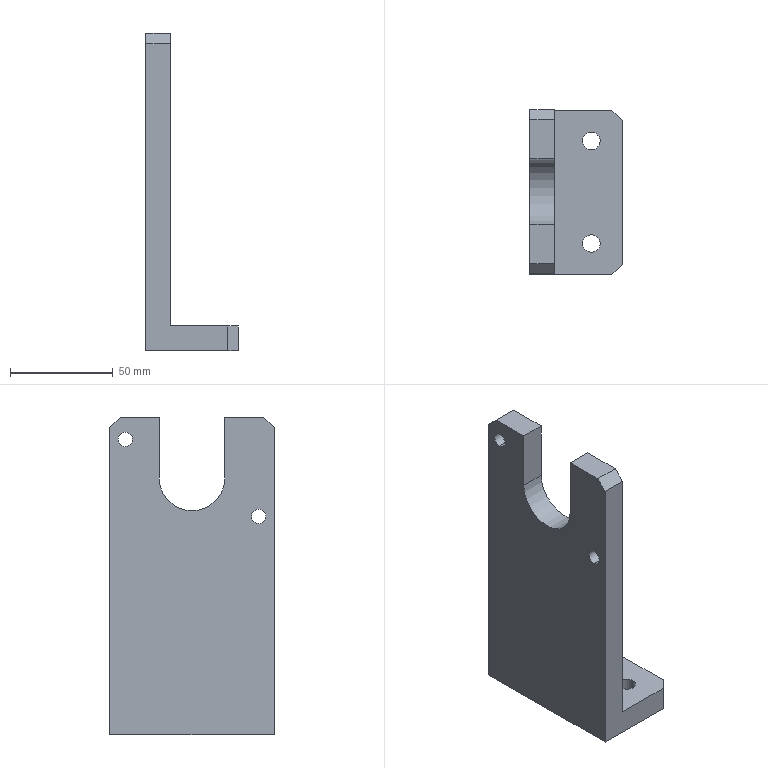Part | SolidWorks | features BaseBody 1 | 1 solid | 24 faces | box 45 x 80 x 154.5 mm | volume 160965 mm3 | plane 15 | cylinder 9 | commonest cylinder face diameters 6.985 x4 8.5 x4 32 x1
STEP:
#1=CARTESIAN_POINT('',(0.,32.476,220.743));
#2=VERTEX_POINT('',#1);
#3=CARTESIAN_POINT('',(0.,32.476,213.757));
#4=VERTEX_POINT('',#3);
#5=CARTESIAN_POINT('',(0.,32.476,217.25));
#6=DIRECTION('',(1.,0.,0.));
#7=DIRECTION('',(0.,0.,1.));
#8=AXIS2_PLACEMENT_3D('',#5,#6,#7);
#9=CIRCLE('',#8,3.493);
#10=EDGE_CURVE('',#2,#4,#9,.T.);
#11=ORIENTED_EDGE('',*,*,#10,.F.);
#12=CARTESIAN_POINT('',(12.,32.476,220.743));
#13=VERTEX_POINT('',#12);
#14=CARTESIAN_POINT('',(0.,32.476,220.743));
#15=DIRECTION('',(1.,0.,0.));
#16=VECTOR('',#15,1000.);
#17=LINE('',#14,#16);
#18=EDGE_CURVE('',#2,#13,#17,.T.);
#19=ORIENTED_EDGE('',*,*,#18,.T.);
#20=CARTESIAN_POINT('',(12.,32.476,213.757));
#21=VERTEX_POINT('',#20);
#22=CARTESIAN_POINT('',(12.,32.476,217.25));
#23=DIRECTION('',(-1.,0.,0.));
#24=DIRECTION('',(0.,0.,-1.));
#25=AXIS2_PLACEMENT_3D('',#22,#23,#24);
#26=CIRCLE('',#25,3.493);
#27=EDGE_CURVE('',#21,#13,#26,.T.);
#28=ORIENTED_EDGE('',*,*,#27,.F.);
#29=CARTESIAN_POINT('',(0.,32.476,213.757));
#30=DIRECTION('',(1.,0.,0.));
#31=VECTOR('',#30,1000.);
#32=LINE('',#29,#31);
#33=EDGE_CURVE('',#4,#21,#32,.T.);
#34=ORIENTED_EDGE('',*,*,#33,.F.);
#35=EDGE_LOOP('',(#11,#19,#28,#34));
#36=FACE_OUTER_BOUND('',#35,.T.);
#37=CARTESIAN_POINT('',(0.,32.476,217.25));
#38=DIRECTION('',(1.,0.,0.));
#39=DIRECTION('',(0.,0.,-1.));
#40=AXIS2_PLACEMENT_3D('',#37,#38,#39);
#41=CYLINDRICAL_SURFACE('',#40,3.493);
#42=ADVANCED_FACE('',(#36),#41,.F.);
#43=CARTESIAN_POINT('',(0.,-32.476,183.243));
#44=VERTEX_POINT('',#43);
#45=CARTESIAN_POINT('',(0.,-32.476,176.257));
#46=VERTEX_POINT('',#45);
#47=CARTESIAN_POINT('',(0.,-32.476,179.75));
#48=DIRECTION('',(1.,0.,0.));
#49=DIRECTION('',(0.,0.,1.));
#50=AXIS2_PLACEMENT_3D('',#47,#48,#49);
#51=CIRCLE('',#50,3.493);
#52=EDGE_CURVE('',#44,#46,#51,.T.);
#53=ORIENTED_EDGE('',*,*,#52,.F.);
#54=CARTESIAN_POINT('',(12.,-32.476,183.243));
#55=VERTEX_POINT('',#54);
#56=CARTESIAN_POINT('',(0.,-32.476,183.243));
#57=DIRECTION('',(1.,0.,0.));
#58=VECTOR('',#57,1000.);
#59=LINE('',#56,#58);
#60=EDGE_CURVE('',#44,#55,#59,.T.);
#61=ORIENTED_EDGE('',*,*,#60,.T.);
#62=CARTESIAN_POINT('',(12.,-32.476,176.257));
#63=VERTEX_POINT('',#62);
#64=CARTESIAN_POINT('',(12.,-32.476,179.75));
#65=DIRECTION('',(-1.,0.,0.));
#66=DIRECTION('',(0.,0.,-1.));
#67=AXIS2_PLACEMENT_3D('',#64,#65,#66);
#68=CIRCLE('',#67,3.493);
#69=EDGE_CURVE('',#63,#55,#68,.T.);
#70=ORIENTED_EDGE('',*,*,#69,.F.);
#71=CARTESIAN_POINT('',(0.,-32.476,176.257));
#72=DIRECTION('',(1.,0.,0.));
#73=VECTOR('',#72,1000.);
#74=LINE('',#71,#73);
#75=EDGE_CURVE('',#46,#63,#74,.T.);
#76=ORIENTED_EDGE('',*,*,#75,.F.);
#77=EDGE_LOOP('',(#53,#61,#70,#76));
#78=FACE_OUTER_BOUND('',#77,.T.);
#79=CARTESIAN_POINT('',(0.,-32.476,179.75));
#80=DIRECTION('',(1.,0.,0.));
#81=DIRECTION('',(0.,0.,-1.));
#82=AXIS2_PLACEMENT_3D('',#79,#80,#81);
#83=CYLINDRICAL_SURFACE('',#82,3.493);
#84=ADVANCED_FACE('',(#78),#83,.F.);
#85=CARTESIAN_POINT('',(34.25,25.,85.5));
#86=VERTEX_POINT('',#85);
#87=CARTESIAN_POINT('',(25.75,25.,85.5));
#88=VERTEX_POINT('',#87);
#89=CARTESIAN_POINT('',(30.,25.,85.5));
#90=DIRECTION('',(0.,0.,-1.));
#91=DIRECTION('',(-1.,0.,0.));
#92=AXIS2_PLACEMENT_3D('',#89,#90,#91);
#93=CIRCLE('',#92,4.25);
#94=EDGE_CURVE('',#86,#88,#93,.T.);
#95=ORIENTED_EDGE('',*,*,#94,.F.);
#96=CARTESIAN_POINT('',(34.25,25.,73.5));
#97=VERTEX_POINT('',#96);
#98=CARTESIAN_POINT('',(34.25,25.,85.5));
#99=DIRECTION('',(0.,0.,-1.));
#100=VECTOR('',#99,1000.);
#101=LINE('',#98,#100);
#102=EDGE_CURVE('',#86,#97,#101,.T.);
#103=ORIENTED_EDGE('',*,*,#102,.T.);
#104=CARTESIAN_POINT('',(25.75,25.,73.5));
#105=VERTEX_POINT('',#104);
#106=CARTESIAN_POINT('',(30.,25.,73.5));
#107=DIRECTION('',(0.,0.,1.));
#108=DIRECTION('',(-1.,0.,0.));
#109=AXIS2_PLACEMENT_3D('',#106,#107,#108);
#110=CIRCLE('',#109,4.25);
#111=EDGE_CURVE('',#105,#97,#110,.T.);
#112=ORIENTED_EDGE('',*,*,#111,.F.);
#113=CARTESIAN_POINT('',(25.75,25.,85.5));
#114=DIRECTION('',(0.,0.,-1.));
#115=VECTOR('',#114,1000.);
#116=LINE('',#113,#115);
#117=EDGE_CURVE('',#88,#105,#116,.T.);
#118=ORIENTED_EDGE('',*,*,#117,.F.);
#119=EDGE_LOOP('',(#95,#103,#112,#118));
#120=FACE_OUTER_BOUND('',#119,.T.);
#121=CARTESIAN_POINT('',(30.,25.,85.5));
#122=DIRECTION('',(0.,0.,-1.));
#123=DIRECTION('',(-1.,0.,0.));
#124=AXIS2_PLACEMENT_3D('',#121,#122,#123);
#125=CYLINDRICAL_SURFACE('',#124,4.25);
#126=ADVANCED_FACE('',(#120),#125,.F.);
#127=CARTESIAN_POINT('',(34.25,-25.,85.5));
#128=VERTEX_POINT('',#127);
#129=CARTESIAN_POINT('',(25.75,-25.,85.5));
#130=VERTEX_POINT('',#129);
#131=CARTESIAN_POINT('',(30.,-25.,85.5));
#132=DIRECTION('',(0.,0.,-1.));
#133=DIRECTION('',(-1.,0.,0.));
#134=AXIS2_PLACEMENT_3D('',#131,#132,#133);
#135=CIRCLE('',#134,4.25);
#136=EDGE_CURVE('',#128,#130,#135,.T.);
#137=ORIENTED_EDGE('',*,*,#136,.F.);
#138=CARTESIAN_POINT('',(34.25,-25.,73.5));
#139=VERTEX_POINT('',#138);
#140=CARTESIAN_POINT('',(34.25,-25.,85.5));
#141=DIRECTION('',(0.,0.,-1.));
#142=VECTOR('',#141,1000.);
#143=LINE('',#140,#142);
#144=EDGE_CURVE('',#128,#139,#143,.T.);
#145=ORIENTED_EDGE('',*,*,#144,.T.);
#146=CARTESIAN_POINT('',(25.75,-25.,73.5));
#147=VERTEX_POINT('',#146);
#148=CARTESIAN_POINT('',(30.,-25.,73.5));
#149=DIRECTION('',(0.,0.,1.));
#150=DIRECTION('',(-1.,0.,0.));
#151=AXIS2_PLACEMENT_3D('',#148,#149,#150);
#152=CIRCLE('',#151,4.25);
#153=EDGE_CURVE('',#147,#139,#152,.T.);
#154=ORIENTED_EDGE('',*,*,#153,.F.);
#155=CARTESIAN_POINT('',(25.75,-25.,85.5));
#156=DIRECTION('',(0.,0.,-1.));
#157=VECTOR('',#156,1000.);
#158=LINE('',#155,#157);
#159=EDGE_CURVE('',#130,#147,#158,.T.);
#160=ORIENTED_EDGE('',*,*,#159,.F.);
#161=EDGE_LOOP('',(#137,#145,#154,#160));
#162=FACE_OUTER_BOUND('',#161,.T.);
#163=CARTESIAN_POINT('',(30.,-25.,85.5));
#164=DIRECTION('',(0.,0.,-1.));
#165=DIRECTION('',(-1.,0.,0.));
#166=AXIS2_PLACEMENT_3D('',#163,#164,#165);
#167=CYLINDRICAL_SURFACE('',#166,4.25);
#168=ADVANCED_FACE('',(#162),#167,.F.);
#169=CARTESIAN_POINT('',(0.,40.,223.));
#170=VERTEX_POINT('',#169);
#171=CARTESIAN_POINT('',(0.,40.,73.5));
#172=VERTEX_POINT('',#171);
#173=CARTESIAN_POINT('',(0.,40.,133.5));
#174=DIRECTION('',(0.,0.,-1.));
#175=VECTOR('',#174,1000.);
#176=LINE('',#173,#175);
#177=EDGE_CURVE('',#170,#172,#176,.T.);
#178=ORIENTED_EDGE('',*,*,#177,.T.);
#179=CARTESIAN_POINT('',(0.,-40.,73.5));
#180=VERTEX_POINT('',#179);
#181=CARTESIAN_POINT('',(0.,-42.5,73.5));
#182=DIRECTION('',(0.,-1.,0.));
#183=VECTOR('',#182,1000.);
#184=LINE('',#181,#183);
#185=EDGE_CURVE('',#172,#180,#184,.T.);
#186=ORIENTED_EDGE('',*,*,#185,.T.);
#187=CARTESIAN_POINT('',(0.,-40.,223.));
#188=VERTEX_POINT('',#187);
#189=CARTESIAN_POINT('',(0.,-40.,133.5));
#190=DIRECTION('',(0.,0.,1.));
#191=VECTOR('',#190,1000.);
#192=LINE('',#189,#191);
#193=EDGE_CURVE('',#180,#188,#192,.T.);
#194=ORIENTED_EDGE('',*,*,#193,.T.);
#195=CARTESIAN_POINT('',(0.,-35.,228.));
#196=VERTEX_POINT('',#195);
#197=CARTESIAN_POINT('',(0.,-84.75,178.25));
#198=DIRECTION('',(0.,0.7071,0.7071));
#199=VECTOR('',#198,1000.);
#200=LINE('',#197,#199);
#201=EDGE_CURVE('',#188,#196,#200,.T.);
#202=ORIENTED_EDGE('',*,*,#201,.T.);
#203=CARTESIAN_POINT('',(0.,-16.,228.));
#204=VERTEX_POINT('',#203);
#205=CARTESIAN_POINT('',(0.,-42.5,228.));
#206=DIRECTION('',(0.,1.,0.));
#207=VECTOR('',#206,1000.);
#208=LINE('',#205,#207);
#209=EDGE_CURVE('',#196,#204,#208,.T.);
#210=ORIENTED_EDGE('',*,*,#209,.T.);
#211=CARTESIAN_POINT('',(0.,-16.,198.5));
#212=VERTEX_POINT('',#211);
#213=CARTESIAN_POINT('',(0.,-16.,133.5));
#214=DIRECTION('',(0.,0.,-1.));
#215=VECTOR('',#214,1000.);
#216=LINE('',#213,#215);
#217=EDGE_CURVE('',#204,#212,#216,.T.);
#218=ORIENTED_EDGE('',*,*,#217,.T.);
#219=CARTESIAN_POINT('',(0.,16.,198.5));
#220=VERTEX_POINT('',#219);
#221=CARTESIAN_POINT('',(0.,0.,198.5));
#222=DIRECTION('',(1.,0.,0.));
#223=DIRECTION('',(0.,0.,1.));
#224=AXIS2_PLACEMENT_3D('',#221,#222,#223);
#225=CIRCLE('',#224,16.);
#226=EDGE_CURVE('',#212,#220,#225,.T.);
#227=ORIENTED_EDGE('',*,*,#226,.T.);
#228=CARTESIAN_POINT('',(0.,16.,228.));
#229=VERTEX_POINT('',#228);
#230=CARTESIAN_POINT('',(0.,16.,133.5));
#231=DIRECTION('',(0.,0.,1.));
#232=VECTOR('',#231,1000.);
#233=LINE('',#230,#232);
#234=EDGE_CURVE('',#220,#229,#233,.T.);
#235=ORIENTED_EDGE('',*,*,#234,.T.);
#236=CARTESIAN_POINT('',(0.,35.,228.));
#237=VERTEX_POINT('',#236);
#238=CARTESIAN_POINT('',(0.,-42.5,228.));
#239=DIRECTION('',(0.,1.,0.));
#240=VECTOR('',#239,1000.);
#241=LINE('',#238,#240);
#242=EDGE_CURVE('',#229,#237,#241,.T.);
#243=ORIENTED_EDGE('',*,*,#242,.T.);
#244=CARTESIAN_POINT('',(0.,40.,223.));
#245=DIRECTION('',(0.,0.7071,-0.7071));
#246=VECTOR('',#245,1000.);
#247=LINE('',#244,#246);
#248=EDGE_CURVE('',#237,#170,#247,.T.);
#249=ORIENTED_EDGE('',*,*,#248,.T.);
#250=EDGE_LOOP('',(#178,#186,#194,#202,#210,#218,#227,#235,#243,#249));
#251=FACE_OUTER_BOUND('',#250,.T.);
#252=CARTESIAN_POINT('',(0.,32.476,217.25));
#253=DIRECTION('',(1.,0.,0.));
#254=DIRECTION('',(0.,0.,1.));
#255=AXIS2_PLACEMENT_3D('',#252,#253,#254);
#256=CIRCLE('',#255,3.493);
#257=EDGE_CURVE('',#4,#2,#256,.T.);
#258=ORIENTED_EDGE('',*,*,#257,.T.);
#259=ORIENTED_EDGE('',*,*,#10,.T.);
#260=EDGE_LOOP('',(#258,#259));
#261=FACE_BOUND('',#260,.T.);
#262=CARTESIAN_POINT('',(0.,-32.476,179.75));
#263=DIRECTION('',(1.,0.,0.));
#264=DIRECTION('',(0.,0.,1.));
#265=AXIS2_PLACEMENT_3D('',#262,#263,#264);
#266=CIRCLE('',#265,3.493);
#267=EDGE_CURVE('',#46,#44,#266,.T.);
#268=ORIENTED_EDGE('',*,*,#267,.T.);
#269=ORIENTED_EDGE('',*,*,#52,.T.);
#270=EDGE_LOOP('',(#268,#269));
#271=FACE_BOUND('',#270,.T.);
#272=CARTESIAN_POINT('',(0.,-42.5,133.5));
#273=DIRECTION('',(-1.,0.,0.));
#274=DIRECTION('',(0.,0.,1.));
#275=AXIS2_PLACEMENT_3D('',#272,#273,#274);
#276=PLANE('',#275);
#277=ADVANCED_FACE('',(#251,#261,#271),#276,.T.);
#278=CARTESIAN_POINT('',(40.,-40.,73.5));
#279=VERTEX_POINT('',#278);
#280=CARTESIAN_POINT('',(0.,-40.,73.5));
#281=DIRECTION('',(-1.,0.,0.));
#282=VECTOR('',#281,1000.);
#283=LINE('',#280,#282);
#284=EDGE_CURVE('',#279,#180,#283,.T.);
#285=ORIENTED_EDGE('',*,*,#284,.T.);
#286=ORIENTED_EDGE('',*,*,#185,.F.);
#287=CARTESIAN_POINT('',(40.,40.,73.5));
#288=VERTEX_POINT('',#287);
#289=CARTESIAN_POINT('',(45.,40.,73.5));
#290=DIRECTION('',(1.,0.,0.));
#291=VECTOR('',#290,1000.);
#292=LINE('',#289,#291);
#293=EDGE_CURVE('',#172,#288,#292,.T.);
#294=ORIENTED_EDGE('',*,*,#293,.T.);
#295=CARTESIAN_POINT('',(45.,35.,73.5));
#296=VERTEX_POINT('',#295);
#297=CARTESIAN_POINT('',(40.,40.,73.5));
#298=DIRECTION('',(0.7071,-0.7071,0.));
#299=VECTOR('',#298,1000.);
#300=LINE('',#297,#299);
#301=EDGE_CURVE('',#288,#296,#300,.T.);
#302=ORIENTED_EDGE('',*,*,#301,.T.);
#303=CARTESIAN_POINT('',(45.,-35.,73.5));
#304=VERTEX_POINT('',#303);
#305=CARTESIAN_POINT('',(45.,-42.5,73.5));
#306=DIRECTION('',(0.,-1.,0.));
#307=VECTOR('',#306,1000.);
#308=LINE('',#305,#307);
#309=EDGE_CURVE('',#296,#304,#308,.T.);
#310=ORIENTED_EDGE('',*,*,#309,.T.);
#311=CARTESIAN_POINT('',(45.,-35.,73.5));
#312=DIRECTION('',(-0.7071,-0.7071,0.));
#313=VECTOR('',#312,1000.);
#314=LINE('',#311,#313);
#315=EDGE_CURVE('',#304,#279,#314,.T.);
#316=ORIENTED_EDGE('',*,*,#315,.T.);
#317=EDGE_LOOP('',(#285,#286,#294,#302,#310,#316));
#318=FACE_OUTER_BOUND('',#317,.T.);
#319=ORIENTED_EDGE('',*,*,#111,.T.);
#320=CARTESIAN_POINT('',(30.,25.,73.5));
#321=DIRECTION('',(0.,0.,1.));
#322=DIRECTION('',(-1.,0.,0.));
#323=AXIS2_PLACEMENT_3D('',#320,#321,#322);
#324=CIRCLE('',#323,4.25);
#325=EDGE_CURVE('',#97,#105,#324,.T.);
#326=ORIENTED_EDGE('',*,*,#325,.T.);
#327=EDGE_LOOP('',(#319,#326));
#328=FACE_BOUND('',#327,.T.);
#329=ORIENTED_EDGE('',*,*,#153,.T.);
#330=CARTESIAN_POINT('',(30.,-25.,73.5));
#331=DIRECTION('',(0.,0.,1.));
#332=DIRECTION('',(-1.,0.,0.));
#333=AXIS2_PLACEMENT_3D('',#330,#331,#332);
#334=CIRCLE('',#333,4.25);
#335=EDGE_CURVE('',#139,#147,#334,.T.);
#336=ORIENTED_EDGE('',*,*,#335,.T.);
#337=EDGE_LOOP('',(#329,#336));
#338=FACE_BOUND('',#337,.T.);
#339=CARTESIAN_POINT('',(45.,-42.5,73.5));
#340=DIRECTION('',(0.,0.,-1.));
#341=DIRECTION('',(-1.,0.,0.));
#342=AXIS2_PLACEMENT_3D('',#339,#340,#341);
#343=PLANE('',#342);
#344=ADVANCED_FACE('',(#318,#328,#338),#343,.T.);
#345=CARTESIAN_POINT('',(12.,40.,223.));
#346=VERTEX_POINT('',#345);
#347=CARTESIAN_POINT('',(0.,40.,223.));
#348=DIRECTION('',(1.,0.,0.));
#349=VECTOR('',#348,1000.);
#350=LINE('',#347,#349);
#351=EDGE_CURVE('',#170,#346,#350,.T.);
#352=ORIENTED_EDGE('',*,*,#351,.T.);
#353=CARTESIAN_POINT('',(12.,40.,85.5));
#354=VERTEX_POINT('',#353);
#355=CARTESIAN_POINT('',(12.,40.,72.));
#356=DIRECTION('',(0.,0.,-1.));
#357=VECTOR('',#356,1000.);
#358=LINE('',#355,#357);
#359=EDGE_CURVE('',#346,#354,#358,.T.);
#360=ORIENTED_EDGE('',*,*,#359,.T.);
#361=CARTESIAN_POINT('',(40.,40.,85.5));
#362=VERTEX_POINT('',#361);
#363=CARTESIAN_POINT('',(0.,40.,85.5));
#364=DIRECTION('',(1.,0.,0.));
#365=VECTOR('',#364,1000.);
#366=LINE('',#363,#365);
#367=EDGE_CURVE('',#354,#362,#366,.T.);
#368=ORIENTED_EDGE('',*,*,#367,.T.);
#369=CARTESIAN_POINT('',(40.,40.,145.5));
#370=DIRECTION('',(0.,0.,-1.));
#371=VECTOR('',#370,1000.);
#372=LINE('',#369,#371);
#373=EDGE_CURVE('',#362,#288,#372,.T.);
#374=ORIENTED_EDGE('',*,*,#373,.T.);
#375=ORIENTED_EDGE('',*,*,#293,.F.);
#376=ORIENTED_EDGE('',*,*,#177,.F.);
#377=EDGE_LOOP('',(#352,#360,#368,#374,#375,#376));
#378=FACE_OUTER_BOUND('',#377,.T.);
#379=CARTESIAN_POINT('',(0.,40.,72.));
#380=DIRECTION('',(0.,1.,0.));
#381=DIRECTION('',(0.,0.,1.));
#382=AXIS2_PLACEMENT_3D('',#379,#380,#381);
#383=PLANE('',#382);
#384=ADVANCED_FACE('',(#378),#383,.T.);
#385=CARTESIAN_POINT('',(12.,35.,228.));
#386=VERTEX_POINT('',#385);
#387=CARTESIAN_POINT('',(0.,35.,228.));
#388=DIRECTION('',(-1.,0.,0.));
#389=VECTOR('',#388,1000.);
#390=LINE('',#387,#389);
#391=EDGE_CURVE('',#386,#237,#390,.T.);
#392=ORIENTED_EDGE('',*,*,#391,.F.);
#393=CARTESIAN_POINT('',(12.,40.,223.));
#394=DIRECTION('',(0.,-0.7071,0.7071));
#395=VECTOR('',#394,1000.);
#396=LINE('',#393,#395);
#397=EDGE_CURVE('',#346,#386,#396,.T.);
#398=ORIENTED_EDGE('',*,*,#397,.F.);
#399=ORIENTED_EDGE('',*,*,#351,.F.);
#400=ORIENTED_EDGE('',*,*,#248,.F.);
#401=EDGE_LOOP('',(#392,#398,#399,#400));
#402=FACE_OUTER_BOUND('',#401,.T.);
#403=CARTESIAN_POINT('',(0.,40.,223.));
#404=DIRECTION('',(0.,-0.7071,-0.7071));
#405=DIRECTION('',(0.,0.7071,-0.7071));
#406=AXIS2_PLACEMENT_3D('',#403,#404,#405);
#407=PLANE('',#406);
#408=ADVANCED_FACE('',(#402),#407,.F.);
#409=ORIENTED_EDGE('',*,*,#242,.F.);
#410=CARTESIAN_POINT('',(12.,16.,228.));
#411=VERTEX_POINT('',#410);
#412=CARTESIAN_POINT('',(0.,16.,228.));
#413=DIRECTION('',(1.,0.,0.));
#414=VECTOR('',#413,1000.);
#415=LINE('',#412,#414);
#416=EDGE_CURVE('',#229,#411,#415,.T.);
#417=ORIENTED_EDGE('',*,*,#416,.T.);
#418=CARTESIAN_POINT('',(12.,-42.5,228.));
#419=DIRECTION('',(0.,1.,0.));
#420=VECTOR('',#419,1000.);
#421=LINE('',#418,#420);
#422=EDGE_CURVE('',#411,#386,#421,.T.);
#423=ORIENTED_EDGE('',*,*,#422,.T.);
#424=ORIENTED_EDGE('',*,*,#391,.T.);
#425=EDGE_LOOP('',(#409,#417,#423,#424));
#426=FACE_OUTER_BOUND('',#425,.T.);
#427=CARTESIAN_POINT('',(0.,-42.5,228.));
#428=DIRECTION('',(0.,0.,1.));
#429=DIRECTION('',(1.,0.,0.));
#430=AXIS2_PLACEMENT_3D('',#427,#428,#429);
#431=PLANE('',#430);
#432=ADVANCED_FACE('',(#426),#431,.T.);
#433=CARTESIAN_POINT('',(12.,16.,198.5));
#434=VERTEX_POINT('',#433);
#435=CARTESIAN_POINT('',(30.,16.,198.5));
#436=DIRECTION('',(1.,0.,0.));
#437=VECTOR('',#436,1000.);
#438=LINE('',#435,#437);
#439=EDGE_CURVE('',#220,#434,#438,.T.);
#440=ORIENTED_EDGE('',*,*,#439,.T.);
#441=CARTESIAN_POINT('',(12.,16.,198.5));
#442=DIRECTION('',(0.,0.,1.));
#443=VECTOR('',#442,1000.);
#444=LINE('',#441,#443);
#445=EDGE_CURVE('',#434,#411,#444,.T.);
#446=ORIENTED_EDGE('',*,*,#445,.T.);
#447=ORIENTED_EDGE('',*,*,#416,.F.);
#448=ORIENTED_EDGE('',*,*,#234,.F.);
#449=EDGE_LOOP('',(#440,#446,#447,#448));
#450=FACE_OUTER_BOUND('',#449,.T.);
#451=CARTESIAN_POINT('',(30.,16.,198.5));
#452=DIRECTION('',(0.,-1.,0.));
#453=DIRECTION('',(0.,0.,-1.));
#454=AXIS2_PLACEMENT_3D('',#451,#452,#453);
#455=PLANE('',#454);
#456=ADVANCED_FACE('',(#450),#455,.T.);
#457=ORIENTED_EDGE('',*,*,#226,.F.);
#458=CARTESIAN_POINT('',(12.,-16.,198.5));
#459=VERTEX_POINT('',#458);
#460=CARTESIAN_POINT('',(30.,-16.,198.5));
#461=DIRECTION('',(-1.,0.,0.));
#462=VECTOR('',#461,1000.);
#463=LINE('',#460,#462);
#464=EDGE_CURVE('',#459,#212,#463,.T.);
#465=ORIENTED_EDGE('',*,*,#464,.F.);
#466=CARTESIAN_POINT('',(12.,0.,198.5));
#467=DIRECTION('',(-1.,0.,0.));
#468=DIRECTION('',(0.,0.,1.));
#469=AXIS2_PLACEMENT_3D('',#466,#467,#468);
#470=CIRCLE('',#469,16.);
#471=EDGE_CURVE('',#434,#459,#470,.T.);
#472=ORIENTED_EDGE('',*,*,#471,.F.);
#473=ORIENTED_EDGE('',*,*,#439,.F.);
#474=EDGE_LOOP('',(#457,#465,#472,#473));
#475=FACE_OUTER_BOUND('',#474,.T.);
#476=CARTESIAN_POINT('',(30.,0.,198.5));
#477=DIRECTION('',(-1.,0.,0.));
#478=DIRECTION('',(0.,0.,1.));
#479=AXIS2_PLACEMENT_3D('',#476,#477,#478);
#480=CYLINDRICAL_SURFACE('',#479,16.);
#481=ADVANCED_FACE('',(#475),#480,.F.);
#482=CARTESIAN_POINT('',(12.,-16.,228.));
#483=VERTEX_POINT('',#482);
#484=CARTESIAN_POINT('',(30.,-16.,228.));
#485=DIRECTION('',(1.,0.,0.));
#486=VECTOR('',#485,1000.);
#487=LINE('',#484,#486);
#488=EDGE_CURVE('',#204,#483,#487,.T.);
#489=ORIENTED_EDGE('',*,*,#488,.T.);
#490=CARTESIAN_POINT('',(12.,-16.,228.));
#491=DIRECTION('',(0.,0.,-1.));
#492=VECTOR('',#491,1000.);
#493=LINE('',#490,#492);
#494=EDGE_CURVE('',#483,#459,#493,.T.);
#495=ORIENTED_EDGE('',*,*,#494,.T.);
#496=ORIENTED_EDGE('',*,*,#464,.T.);
#497=ORIENTED_EDGE('',*,*,#217,.F.);
#498=EDGE_LOOP('',(#489,#495,#496,#497));
#499=FACE_OUTER_BOUND('',#498,.T.);
#500=CARTESIAN_POINT('',(30.,-16.,228.));
#501=DIRECTION('',(0.,1.,0.));
#502=DIRECTION('',(0.,0.,1.));
#503=AXIS2_PLACEMENT_3D('',#500,#501,#502);
#504=PLANE('',#503);
#505=ADVANCED_FACE('',(#499),#504,.T.);
#506=CARTESIAN_POINT('',(12.,-35.,228.));
#507=VERTEX_POINT('',#506);
#508=CARTESIAN_POINT('',(12.,-42.5,228.));
#509=DIRECTION('',(0.,1.,0.));
#510=VECTOR('',#509,1000.);
#511=LINE('',#508,#510);
#512=EDGE_CURVE('',#507,#483,#511,.T.);
#513=ORIENTED_EDGE('',*,*,#512,.T.);
#514=ORIENTED_EDGE('',*,*,#488,.F.);
#515=ORIENTED_EDGE('',*,*,#209,.F.);
#516=CARTESIAN_POINT('',(0.,-35.,228.));
#517=DIRECTION('',(1.,0.,0.));
#518=VECTOR('',#517,1000.);
#519=LINE('',#516,#518);
#520=EDGE_CURVE('',#196,#507,#519,.T.);
#521=ORIENTED_EDGE('',*,*,#520,.T.);
#522=EDGE_LOOP('',(#513,#514,#515,#521));
#523=FACE_OUTER_BOUND('',#522,.T.);
#524=CARTESIAN_POINT('',(0.,-42.5,228.));
#525=DIRECTION('',(0.,0.,1.));
#526=DIRECTION('',(1.,0.,0.));
#527=AXIS2_PLACEMENT_3D('',#524,#525,#526);
#528=PLANE('',#527);
#529=ADVANCED_FACE('',(#523),#528,.T.);
#530=CARTESIAN_POINT('',(12.,-40.,223.));
#531=VERTEX_POINT('',#530);
#532=CARTESIAN_POINT('',(12.,-35.,228.));
#533=DIRECTION('',(0.,0.7071,0.7071));
#534=VECTOR('',#533,1000.);
#535=LINE('',#532,#534);
#536=EDGE_CURVE('',#531,#507,#535,.T.);
#537=ORIENTED_EDGE('',*,*,#536,.T.);
#538=ORIENTED_EDGE('',*,*,#520,.F.);
#539=ORIENTED_EDGE('',*,*,#201,.F.);
#540=CARTESIAN_POINT('',(0.,-40.,223.));
#541=DIRECTION('',(1.,0.,0.));
#542=VECTOR('',#541,1000.);
#543=LINE('',#540,#542);
#544=EDGE_CURVE('',#188,#531,#543,.T.);
#545=ORIENTED_EDGE('',*,*,#544,.T.);
#546=EDGE_LOOP('',(#537,#538,#539,#545));
#547=FACE_OUTER_BOUND('',#546,.T.);
#548=CARTESIAN_POINT('',(0.,-35.,228.));
#549=DIRECTION('',(0.,-0.7071,0.7071));
#550=DIRECTION('',(0.,-0.7071,-0.7071));
#551=AXIS2_PLACEMENT_3D('',#548,#549,#550);
#552=PLANE('',#551);
#553=ADVANCED_FACE('',(#547),#552,.T.);
#554=CARTESIAN_POINT('',(40.,-40.,85.5));
#555=VERTEX_POINT('',#554);
#556=CARTESIAN_POINT('',(40.,-40.,135.5));
#557=DIRECTION('',(0.,0.,-1.));
#558=VECTOR('',#557,1000.);
#559=LINE('',#556,#558);
#560=EDGE_CURVE('',#555,#279,#559,.T.);
#561=ORIENTED_EDGE('',*,*,#560,.F.);
#562=CARTESIAN_POINT('',(12.,-40.,85.5));
#563=VERTEX_POINT('',#562);
#564=CARTESIAN_POINT('',(0.,-40.,85.5));
#565=DIRECTION('',(1.,0.,0.));
#566=VECTOR('',#565,1000.);
#567=LINE('',#564,#566);
#568=EDGE_CURVE('',#563,#555,#567,.T.);
#569=ORIENTED_EDGE('',*,*,#568,.F.);
#570=CARTESIAN_POINT('',(12.,-40.,145.5));
#571=DIRECTION('',(0.,0.,-1.));
#572=VECTOR('',#571,1000.);
#573=LINE('',#570,#572);
#574=EDGE_CURVE('',#531,#563,#573,.T.);
#575=ORIENTED_EDGE('',*,*,#574,.F.);
#576=ORIENTED_EDGE('',*,*,#544,.F.);
#577=ORIENTED_EDGE('',*,*,#193,.F.);
#578=ORIENTED_EDGE('',*,*,#284,.F.);
#579=EDGE_LOOP('',(#561,#569,#575,#576,#577,#578));
#580=FACE_OUTER_BOUND('',#579,.T.);
#581=CARTESIAN_POINT('',(0.,-40.,135.5));
#582=DIRECTION('',(0.,1.,0.));
#583=DIRECTION('',(0.,0.,1.));
#584=AXIS2_PLACEMENT_3D('',#581,#582,#583);
#585=PLANE('',#584);
#586=ADVANCED_FACE('',(#580),#585,.F.);
#587=ORIENTED_EDGE('',*,*,#18,.F.);
#588=ORIENTED_EDGE('',*,*,#257,.F.);
#589=ORIENTED_EDGE('',*,*,#33,.T.);
#590=CARTESIAN_POINT('',(12.,32.476,217.25));
#591=DIRECTION('',(-1.,0.,0.));
#592=DIRECTION('',(0.,0.,-1.));
#593=AXIS2_PLACEMENT_3D('',#590,#591,#592);
#594=CIRCLE('',#593,3.493);
#595=EDGE_CURVE('',#13,#21,#594,.T.);
#596=ORIENTED_EDGE('',*,*,#595,.F.);
#597=EDGE_LOOP('',(#587,#588,#589,#596));
#598=FACE_OUTER_BOUND('',#597,.T.);
#599=CARTESIAN_POINT('',(0.,32.476,217.25));
#600=DIRECTION('',(1.,0.,0.));
#601=DIRECTION('',(0.,0.,-1.));
#602=AXIS2_PLACEMENT_3D('',#599,#600,#601);
#603=CYLINDRICAL_SURFACE('',#602,3.493);
#604=ADVANCED_FACE('',(#598),#603,.F.);
#605=ORIENTED_EDGE('',*,*,#60,.F.);
#606=ORIENTED_EDGE('',*,*,#267,.F.);
#607=ORIENTED_EDGE('',*,*,#75,.T.);
#608=CARTESIAN_POINT('',(12.,-32.476,179.75));
#609=DIRECTION('',(-1.,0.,0.));
#610=DIRECTION('',(0.,0.,-1.));
#611=AXIS2_PLACEMENT_3D('',#608,#609,#610);
#612=CIRCLE('',#611,3.493);
#613=EDGE_CURVE('',#55,#63,#612,.T.);
#614=ORIENTED_EDGE('',*,*,#613,.F.);
#615=EDGE_LOOP('',(#605,#606,#607,#614));
#616=FACE_OUTER_BOUND('',#615,.T.);
#617=CARTESIAN_POINT('',(0.,-32.476,179.75));
#618=DIRECTION('',(1.,0.,0.));
#619=DIRECTION('',(0.,0.,-1.));
#620=AXIS2_PLACEMENT_3D('',#617,#618,#619);
#621=CYLINDRICAL_SURFACE('',#620,3.493);
#622=ADVANCED_FACE('',(#616),#621,.F.);
#623=ORIENTED_EDGE('',*,*,#315,.F.);
#624=CARTESIAN_POINT('',(45.,-35.,85.5));
#625=VERTEX_POINT('',#624);
#626=CARTESIAN_POINT('',(45.,-35.,85.5));
#627=DIRECTION('',(0.,0.,1.));
#628=VECTOR('',#627,1000.);
#629=LINE('',#626,#628);
#630=EDGE_CURVE('',#304,#625,#629,.T.);
#631=ORIENTED_EDGE('',*,*,#630,.T.);
#632=CARTESIAN_POINT('',(45.,-35.,85.5));
#633=DIRECTION('',(-0.7071,-0.7071,0.));
#634=VECTOR('',#633,1000.);
#635=LINE('',#632,#634);
#636=EDGE_CURVE('',#625,#555,#635,.T.);
#637=ORIENTED_EDGE('',*,*,#636,.T.);
#638=ORIENTED_EDGE('',*,*,#560,.T.);
#639=EDGE_LOOP('',(#623,#631,#637,#638));
#640=FACE_OUTER_BOUND('',#639,.T.);
#641=CARTESIAN_POINT('',(45.,-35.,85.5));
#642=DIRECTION('',(0.7071,-0.7071,0.));
#643=DIRECTION('',(0.7071,0.7071,0.));
#644=AXIS2_PLACEMENT_3D('',#641,#642,#643);
#645=PLANE('',#644);
#646=ADVANCED_FACE('',(#640),#645,.T.);
#647=CARTESIAN_POINT('',(45.,35.,85.5));
#648=VERTEX_POINT('',#647);
#649=CARTESIAN_POINT('',(45.,-42.5,85.5));
#650=DIRECTION('',(0.,-1.,0.));
#651=VECTOR('',#650,1000.);
#652=LINE('',#649,#651);
#653=EDGE_CURVE('',#648,#625,#652,.T.);
#654=ORIENTED_EDGE('',*,*,#653,.T.);
#655=ORIENTED_EDGE('',*,*,#630,.F.);
#656=ORIENTED_EDGE('',*,*,#309,.F.);
#657=CARTESIAN_POINT('',(45.,35.,85.5));
#658=DIRECTION('',(0.,0.,1.));
#659=VECTOR('',#658,1000.);
#660=LINE('',#657,#659);
#661=EDGE_CURVE('',#296,#648,#660,.T.);
#662=ORIENTED_EDGE('',*,*,#661,.T.);
#663=EDGE_LOOP('',(#654,#655,#656,#662));
#664=FACE_OUTER_BOUND('',#663,.T.);
#665=CARTESIAN_POINT('',(45.,-42.5,85.5));
#666=DIRECTION('',(1.,0.,0.));
#667=DIRECTION('',(0.,0.,-1.));
#668=AXIS2_PLACEMENT_3D('',#665,#666,#667);
#669=PLANE('',#668);
#670=ADVANCED_FACE('',(#664),#669,.T.);
#671=ORIENTED_EDGE('',*,*,#661,.F.);
#672=ORIENTED_EDGE('',*,*,#301,.F.);
#673=ORIENTED_EDGE('',*,*,#373,.F.);
#674=CARTESIAN_POINT('',(40.,40.,85.5));
#675=DIRECTION('',(-0.7071,0.7071,0.));
#676=VECTOR('',#675,1000.);
#677=LINE('',#674,#676);
#678=EDGE_CURVE('',#648,#362,#677,.T.);
#679=ORIENTED_EDGE('',*,*,#678,.F.);
#680=EDGE_LOOP('',(#671,#672,#673,#679));
#681=FACE_OUTER_BOUND('',#680,.T.);
#682=CARTESIAN_POINT('',(40.,40.,85.5));
#683=DIRECTION('',(-0.7071,-0.7071,0.));
#684=DIRECTION('',(0.7071,-0.7071,0.));
#685=AXIS2_PLACEMENT_3D('',#682,#683,#684);
#686=PLANE('',#685);
#687=ADVANCED_FACE('',(#681),#686,.F.);
#688=ORIENTED_EDGE('',*,*,#102,.F.);
#689=CARTESIAN_POINT('',(30.,25.,85.5));
#690=DIRECTION('',(0.,0.,-1.));
#691=DIRECTION('',(-1.,0.,0.));
#692=AXIS2_PLACEMENT_3D('',#689,#690,#691);
#693=CIRCLE('',#692,4.25);
#694=EDGE_CURVE('',#88,#86,#693,.T.);
#695=ORIENTED_EDGE('',*,*,#694,.F.);
#696=ORIENTED_EDGE('',*,*,#117,.T.);
#697=ORIENTED_EDGE('',*,*,#325,.F.);
#698=EDGE_LOOP('',(#688,#695,#696,#697));
#699=FACE_OUTER_BOUND('',#698,.T.);
#700=CARTESIAN_POINT('',(30.,25.,85.5));
#701=DIRECTION('',(0.,0.,-1.));
#702=DIRECTION('',(-1.,0.,0.));
#703=AXIS2_PLACEMENT_3D('',#700,#701,#702);
#704=CYLINDRICAL_SURFACE('',#703,4.25);
#705=ADVANCED_FACE('',(#699),#704,.F.);
#706=ORIENTED_EDGE('',*,*,#144,.F.);
#707=CARTESIAN_POINT('',(30.,-25.,85.5));
#708=DIRECTION('',(0.,0.,-1.));
#709=DIRECTION('',(-1.,0.,0.));
#710=AXIS2_PLACEMENT_3D('',#707,#708,#709);
#711=CIRCLE('',#710,4.25);
#712=EDGE_CURVE('',#130,#128,#711,.T.);
#713=ORIENTED_EDGE('',*,*,#712,.F.);
#714=ORIENTED_EDGE('',*,*,#159,.T.);
#715=ORIENTED_EDGE('',*,*,#335,.F.);
#716=EDGE_LOOP('',(#706,#713,#714,#715));
#717=FACE_OUTER_BOUND('',#716,.T.);
#718=CARTESIAN_POINT('',(30.,-25.,85.5));
#719=DIRECTION('',(0.,0.,-1.));
#720=DIRECTION('',(-1.,0.,0.));
#721=AXIS2_PLACEMENT_3D('',#718,#719,#720);
#722=CYLINDRICAL_SURFACE('',#721,4.25);
#723=ADVANCED_FACE('',(#717),#722,.F.);
#724=ORIENTED_EDGE('',*,*,#471,.T.);
#725=ORIENTED_EDGE('',*,*,#494,.F.);
#726=ORIENTED_EDGE('',*,*,#512,.F.);
#727=ORIENTED_EDGE('',*,*,#536,.F.);
#728=ORIENTED_EDGE('',*,*,#574,.T.);
#729=CARTESIAN_POINT('',(12.,-42.5,85.5));
#730=DIRECTION('',(0.,1.,0.));
#731=VECTOR('',#730,1000.);
#732=LINE('',#729,#731);
#733=EDGE_CURVE('',#563,#354,#732,.T.);
#734=ORIENTED_EDGE('',*,*,#733,.T.);
#735=ORIENTED_EDGE('',*,*,#359,.F.);
#736=ORIENTED_EDGE('',*,*,#397,.T.);
#737=ORIENTED_EDGE('',*,*,#422,.F.);
#738=ORIENTED_EDGE('',*,*,#445,.F.);
#739=EDGE_LOOP('',(#724,#725,#726,#727,#728,#734,#735,#736,#737,#738));
#740=FACE_OUTER_BOUND('',#739,.T.);
#741=ORIENTED_EDGE('',*,*,#27,.T.);
#742=ORIENTED_EDGE('',*,*,#595,.T.);
#743=EDGE_LOOP('',(#741,#742));
#744=FACE_BOUND('',#743,.T.);
#745=ORIENTED_EDGE('',*,*,#69,.T.);
#746=ORIENTED_EDGE('',*,*,#613,.T.);
#747=EDGE_LOOP('',(#745,#746));
#748=FACE_BOUND('',#747,.T.);
#749=CARTESIAN_POINT('',(12.,-42.5,228.));
#750=DIRECTION('',(1.,0.,0.));
#751=DIRECTION('',(0.,0.,-1.));
#752=AXIS2_PLACEMENT_3D('',#749,#750,#751);
#753=PLANE('',#752);
#754=ADVANCED_FACE('',(#740,#744,#748),#753,.T.);
#755=ORIENTED_EDGE('',*,*,#568,.T.);
#756=ORIENTED_EDGE('',*,*,#636,.F.);
#757=ORIENTED_EDGE('',*,*,#653,.F.);
#758=ORIENTED_EDGE('',*,*,#678,.T.);
#759=ORIENTED_EDGE('',*,*,#367,.F.);
#760=ORIENTED_EDGE('',*,*,#733,.F.);
#761=EDGE_LOOP('',(#755,#756,#757,#758,#759,#760));
#762=FACE_OUTER_BOUND('',#761,.T.);
#763=ORIENTED_EDGE('',*,*,#694,.T.);
#764=ORIENTED_EDGE('',*,*,#94,.T.);
#765=EDGE_LOOP('',(#763,#764));
#766=FACE_BOUND('',#765,.T.);
#767=ORIENTED_EDGE('',*,*,#712,.T.);
#768=ORIENTED_EDGE('',*,*,#136,.T.);
#769=EDGE_LOOP('',(#767,#768));
#770=FACE_BOUND('',#769,.T.);
#771=CARTESIAN_POINT('',(12.,-42.5,85.5));
#772=DIRECTION('',(0.,0.,1.));
#773=DIRECTION('',(1.,0.,0.));
#774=AXIS2_PLACEMENT_3D('',#771,#772,#773);
#775=PLANE('',#774);
#776=ADVANCED_FACE('',(#762,#766,#770),#775,.T.);
#777=CLOSED_SHELL('',(#42,#84,#126,#168,#277,#344,#384,#408,#432,#456,#481,#505,#529,#553,#586,#604,#622,#646,#670,#687,#705,#723,#754,#776));
#778=MANIFOLD_SOLID_BREP('',#777);
#779=CARTESIAN_POINT('',(0.,0.,0.));
#780=DIRECTION('',(0.,0.,1.));
#781=DIRECTION('',(1.,0.,0.));
#782=AXIS2_PLACEMENT_3D('',#779,#780,#781);
#783=(LENGTH_UNIT()NAMED_UNIT(*)SI_UNIT(.MILLI.,.METRE.));
#784=UNCERTAINTY_MEASURE_WITH_UNIT(LENGTH_MEASURE(0.00001),#783,'','');
#785=(NAMED_UNIT(*)PLANE_ANGLE_UNIT()SI_UNIT($,.RADIAN.));
#786=(NAMED_UNIT(*)SI_UNIT($,.STERADIAN.)SOLID_ANGLE_UNIT());
#787=(GEOMETRIC_REPRESENTATION_CONTEXT(3)GLOBAL_UNCERTAINTY_ASSIGNED_CONTEXT((#784))GLOBAL_UNIT_ASSIGNED_CONTEXT((#783,#785,#786))REPRESENTATION_CONTEXT('',''));
#788=ADVANCED_BREP_SHAPE_REPRESENTATION('',(#778,#782),#787);